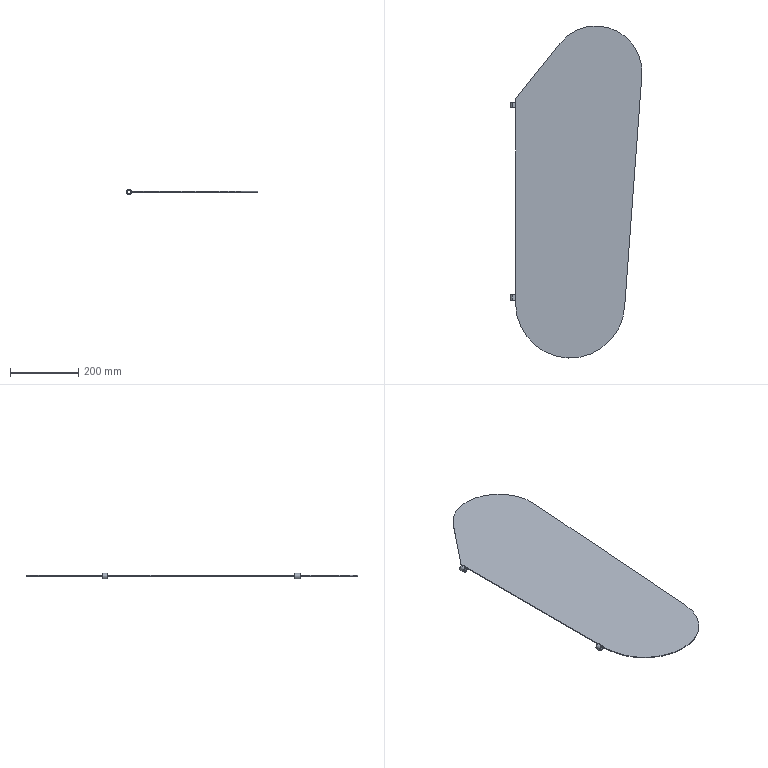Part | SolidWorks | features ICE 3, Extrusion 1, WeldmentFeature 1 | 3 solids | 19 faces | box 386.5 x 973.632 x 16 mm | volume 607839 mm3 | cylinder 10 | plane 9 | commonest cylinder face diameters 10 x4 16 x4 270 x1 320 x1
STEP:
#1=CARTESIAN_POINT('',(-185.,-325.,0.));
#2=VERTEX_POINT('',#1);
#3=CARTESIAN_POINT('',(134.56,-336.857,0.));
#4=VERTEX_POINT('',#3);
#5=CARTESIAN_POINT('',(-25.,-325.,0.));
#6=DIRECTION('',(0.,0.,1.));
#7=DIRECTION('',(1.,0.,0.));
#8=AXIS2_PLACEMENT_3D('',#5,#6,#7);
#9=CIRCLE('',#8,160.);
#10=EDGE_CURVE('',#2,#4,#9,.T.);
#11=ORIENTED_EDGE('',*,*,#10,.T.);
#12=CARTESIAN_POINT('',(134.56,-336.857,2.));
#13=VERTEX_POINT('',#12);
#14=CARTESIAN_POINT('',(134.56,-336.857,2.));
#15=DIRECTION('',(0.,0.,-1.));
#16=VECTOR('',#15,1000.);
#17=LINE('',#14,#16);
#18=EDGE_CURVE('',#13,#4,#17,.T.);
#19=ORIENTED_EDGE('',*,*,#18,.F.);
#20=CARTESIAN_POINT('',(-185.,-325.,2.));
#21=VERTEX_POINT('',#20);
#22=CARTESIAN_POINT('',(-25.,-325.,2.));
#23=DIRECTION('',(0.,0.,1.));
#24=DIRECTION('',(1.,0.,0.));
#25=AXIS2_PLACEMENT_3D('',#22,#23,#24);
#26=CIRCLE('',#25,160.);
#27=EDGE_CURVE('',#21,#13,#26,.T.);
#28=ORIENTED_EDGE('',*,*,#27,.F.);
#29=CARTESIAN_POINT('',(-185.,-325.,2.));
#30=DIRECTION('',(0.,0.,-1.));
#31=VECTOR('',#30,1000.);
#32=LINE('',#29,#31);
#33=EDGE_CURVE('',#21,#2,#32,.T.);
#34=ORIENTED_EDGE('',*,*,#33,.T.);
#35=EDGE_LOOP('',(#11,#19,#28,#34));
#36=FACE_OUTER_BOUND('',#35,.T.);
#37=CARTESIAN_POINT('',(-25.,-325.,2.));
#38=DIRECTION('',(0.,0.,-1.));
#39=DIRECTION('',(-1.,0.,0.));
#40=AXIS2_PLACEMENT_3D('',#37,#38,#39);
#41=CYLINDRICAL_SURFACE('',#40,160.);
#42=ADVANCED_FACE('',(#36),#41,.T.);
#43=CARTESIAN_POINT('',(185.129,343.627,0.));
#44=VERTEX_POINT('',#43);
#45=CARTESIAN_POINT('',(134.56,-336.857,0.));
#46=DIRECTION('',(0.07411,0.9973,0.));
#47=VECTOR('',#46,1000.);
#48=LINE('',#45,#47);
#49=EDGE_CURVE('',#4,#44,#48,.T.);
#50=ORIENTED_EDGE('',*,*,#49,.T.);
#51=CARTESIAN_POINT('',(185.129,343.627,2.));
#52=VERTEX_POINT('',#51);
#53=CARTESIAN_POINT('',(185.129,343.627,2.));
#54=DIRECTION('',(0.,0.,-1.));
#55=VECTOR('',#54,1000.);
#56=LINE('',#53,#55);
#57=EDGE_CURVE('',#52,#44,#56,.T.);
#58=ORIENTED_EDGE('',*,*,#57,.F.);
#59=CARTESIAN_POINT('',(134.56,-336.857,2.));
#60=DIRECTION('',(0.07411,0.9973,0.));
#61=VECTOR('',#60,1000.);
#62=LINE('',#59,#61);
#63=EDGE_CURVE('',#13,#52,#62,.T.);
#64=ORIENTED_EDGE('',*,*,#63,.F.);
#65=ORIENTED_EDGE('',*,*,#18,.T.);
#66=EDGE_LOOP('',(#50,#58,#64,#65));
#67=FACE_OUTER_BOUND('',#66,.T.);
#68=CARTESIAN_POINT('',(134.56,-336.857,2.));
#69=DIRECTION('',(-0.9973,0.07411,0.));
#70=DIRECTION('',(-0.07411,-0.9973,0.));
#71=AXIS2_PLACEMENT_3D('',#68,#69,#70);
#72=PLANE('',#71);
#73=ADVANCED_FACE('',(#67),#72,.F.);
#74=CARTESIAN_POINT('',(-55.009,437.851,0.));
#75=VERTEX_POINT('',#74);
#76=CARTESIAN_POINT('',(50.5,353.632,0.));
#77=DIRECTION('',(0.,0.,1.));
#78=DIRECTION('',(1.,0.,0.));
#79=AXIS2_PLACEMENT_3D('',#76,#77,#78);
#80=CIRCLE('',#79,135.);
#81=EDGE_CURVE('',#44,#75,#80,.T.);
#82=ORIENTED_EDGE('',*,*,#81,.T.);
#83=CARTESIAN_POINT('',(-55.009,437.851,2.));
#84=VERTEX_POINT('',#83);
#85=CARTESIAN_POINT('',(-55.009,437.851,2.));
#86=DIRECTION('',(0.,0.,-1.));
#87=VECTOR('',#86,1000.);
#88=LINE('',#85,#87);
#89=EDGE_CURVE('',#84,#75,#88,.T.);
#90=ORIENTED_EDGE('',*,*,#89,.F.);
#91=CARTESIAN_POINT('',(50.5,353.632,2.));
#92=DIRECTION('',(0.,0.,1.));
#93=DIRECTION('',(1.,0.,0.));
#94=AXIS2_PLACEMENT_3D('',#91,#92,#93);
#95=CIRCLE('',#94,135.);
#96=EDGE_CURVE('',#52,#84,#95,.T.);
#97=ORIENTED_EDGE('',*,*,#96,.F.);
#98=ORIENTED_EDGE('',*,*,#57,.T.);
#99=EDGE_LOOP('',(#82,#90,#97,#98));
#100=FACE_OUTER_BOUND('',#99,.T.);
#101=CARTESIAN_POINT('',(50.5,353.632,2.));
#102=DIRECTION('',(0.,0.,-1.));
#103=DIRECTION('',(-1.,0.,0.));
#104=AXIS2_PLACEMENT_3D('',#101,#102,#103);
#105=CYLINDRICAL_SURFACE('',#104,135.);
#106=ADVANCED_FACE('',(#100),#105,.T.);
#107=CARTESIAN_POINT('',(-185.,275.,0.));
#108=VERTEX_POINT('',#107);
#109=CARTESIAN_POINT('',(-55.009,437.851,0.));
#110=DIRECTION('',(-0.6238,-0.7815,0.));
#111=VECTOR('',#110,1000.);
#112=LINE('',#109,#111);
#113=EDGE_CURVE('',#75,#108,#112,.T.);
#114=ORIENTED_EDGE('',*,*,#113,.T.);
#115=CARTESIAN_POINT('',(-185.,275.,2.));
#116=VERTEX_POINT('',#115);
#117=CARTESIAN_POINT('',(-185.,275.,2.));
#118=DIRECTION('',(0.,0.,-1.));
#119=VECTOR('',#118,1000.);
#120=LINE('',#117,#119);
#121=EDGE_CURVE('',#116,#108,#120,.T.);
#122=ORIENTED_EDGE('',*,*,#121,.F.);
#123=CARTESIAN_POINT('',(-55.009,437.851,2.));
#124=DIRECTION('',(-0.6238,-0.7815,0.));
#125=VECTOR('',#124,1000.);
#126=LINE('',#123,#125);
#127=EDGE_CURVE('',#84,#116,#126,.T.);
#128=ORIENTED_EDGE('',*,*,#127,.F.);
#129=ORIENTED_EDGE('',*,*,#89,.T.);
#130=EDGE_LOOP('',(#114,#122,#128,#129));
#131=FACE_OUTER_BOUND('',#130,.T.);
#132=CARTESIAN_POINT('',(-55.009,437.851,2.));
#133=DIRECTION('',(0.7815,-0.6238,0.));
#134=DIRECTION('',(0.6238,0.7815,0.));
#135=AXIS2_PLACEMENT_3D('',#132,#133,#134);
#136=PLANE('',#135);
#137=ADVANCED_FACE('',(#131),#136,.F.);
#138=CARTESIAN_POINT('',(-185.,275.,0.));
#139=DIRECTION('',(0.,-1.,0.));
#140=VECTOR('',#139,1000.);
#141=LINE('',#138,#140);
#142=EDGE_CURVE('',#108,#2,#141,.T.);
#143=ORIENTED_EDGE('',*,*,#142,.T.);
#144=ORIENTED_EDGE('',*,*,#33,.F.);
#145=CARTESIAN_POINT('',(-185.,275.,2.));
#146=DIRECTION('',(0.,-1.,0.));
#147=VECTOR('',#146,1000.);
#148=LINE('',#145,#147);
#149=EDGE_CURVE('',#116,#21,#148,.T.);
#150=ORIENTED_EDGE('',*,*,#149,.F.);
#151=ORIENTED_EDGE('',*,*,#121,.T.);
#152=EDGE_LOOP('',(#143,#144,#150,#151));
#153=FACE_OUTER_BOUND('',#152,.T.);
#154=CARTESIAN_POINT('',(-185.,275.,2.));
#155=DIRECTION('',(1.,0.,0.));
#156=DIRECTION('',(0.,0.,-1.));
#157=AXIS2_PLACEMENT_3D('',#154,#155,#156);
#158=PLANE('',#157);
#159=ADVANCED_FACE('',(#153),#158,.F.);
#160=ORIENTED_EDGE('',*,*,#27,.T.);
#161=ORIENTED_EDGE('',*,*,#63,.T.);
#162=ORIENTED_EDGE('',*,*,#96,.T.);
#163=ORIENTED_EDGE('',*,*,#127,.T.);
#164=ORIENTED_EDGE('',*,*,#149,.T.);
#165=EDGE_LOOP('',(#160,#161,#162,#163,#164));
#166=FACE_OUTER_BOUND('',#165,.T.);
#167=CARTESIAN_POINT('',(-25.,-325.,2.));
#168=DIRECTION('',(0.,0.,1.));
#169=DIRECTION('',(1.,0.,0.));
#170=AXIS2_PLACEMENT_3D('',#167,#168,#169);
#171=PLANE('',#170);
#172=ADVANCED_FACE('',(#166),#171,.T.);
#173=ORIENTED_EDGE('',*,*,#10,.F.);
#174=ORIENTED_EDGE('',*,*,#142,.F.);
#175=ORIENTED_EDGE('',*,*,#113,.F.);
#176=ORIENTED_EDGE('',*,*,#81,.F.);
#177=ORIENTED_EDGE('',*,*,#49,.F.);
#178=EDGE_LOOP('',(#173,#174,#175,#176,#177));
#179=FACE_OUTER_BOUND('',#178,.T.);
#180=CARTESIAN_POINT('',(-25.,-325.,0.));
#181=DIRECTION('',(0.,0.,1.));
#182=DIRECTION('',(1.,0.,0.));
#183=AXIS2_PLACEMENT_3D('',#180,#181,#182);
#184=PLANE('',#183);
#185=ADVANCED_FACE('',(#179),#184,.F.);
#186=CLOSED_SHELL('',(#42,#73,#106,#137,#159,#172,#185));
#187=MANIFOLD_SOLID_BREP('',#186);
#188=CARTESIAN_POINT('',(-193.,-315.,-5.));
#189=VERTEX_POINT('',#188);
#190=CARTESIAN_POINT('',(-193.,-315.,5.));
#191=VERTEX_POINT('',#190);
#192=CARTESIAN_POINT('',(-193.,-315.,0.));
#193=DIRECTION('',(0.,1.,0.));
#194=DIRECTION('',(0.,0.,1.));
#195=AXIS2_PLACEMENT_3D('',#192,#193,#194);
#196=CIRCLE('',#195,5.);
#197=EDGE_CURVE('',#189,#191,#196,.T.);
#198=ORIENTED_EDGE('',*,*,#197,.F.);
#199=CARTESIAN_POINT('',(-193.,-300.,-5.));
#200=VERTEX_POINT('',#199);
#201=CARTESIAN_POINT('',(-193.,-485.,-5.));
#202=DIRECTION('',(0.,1.,0.));
#203=VECTOR('',#202,1000.);
#204=LINE('',#201,#203);
#205=EDGE_CURVE('',#189,#200,#204,.T.);
#206=ORIENTED_EDGE('',*,*,#205,.T.);
#207=CARTESIAN_POINT('',(-193.,-300.,5.));
#208=VERTEX_POINT('',#207);
#209=CARTESIAN_POINT('',(-193.,-300.,0.));
#210=DIRECTION('',(0.,1.,0.));
#211=DIRECTION('',(0.,0.,1.));
#212=AXIS2_PLACEMENT_3D('',#209,#210,#211);
#213=CIRCLE('',#212,5.);
#214=EDGE_CURVE('',#200,#208,#213,.T.);
#215=ORIENTED_EDGE('',*,*,#214,.T.);
#216=CARTESIAN_POINT('',(-193.,-485.,5.));
#217=DIRECTION('',(0.,1.,0.));
#218=VECTOR('',#217,1000.);
#219=LINE('',#216,#218);
#220=EDGE_CURVE('',#191,#208,#219,.T.);
#221=ORIENTED_EDGE('',*,*,#220,.F.);
#222=EDGE_LOOP('',(#198,#206,#215,#221));
#223=FACE_OUTER_BOUND('',#222,.T.);
#224=CARTESIAN_POINT('',(-193.,-485.,0.));
#225=DIRECTION('',(0.,1.,0.));
#226=DIRECTION('',(0.,0.,1.));
#227=AXIS2_PLACEMENT_3D('',#224,#225,#226);
#228=CYLINDRICAL_SURFACE('',#227,5.);
#229=ADVANCED_FACE('',(#223),#228,.F.);
#230=CARTESIAN_POINT('',(-193.,-300.,8.));
#231=VERTEX_POINT('',#230);
#232=CARTESIAN_POINT('',(-193.,-300.,-8.));
#233=VERTEX_POINT('',#232);
#234=CARTESIAN_POINT('',(-193.,-300.,0.));
#235=DIRECTION('',(0.,1.,0.));
#236=DIRECTION('',(0.,0.,1.));
#237=AXIS2_PLACEMENT_3D('',#234,#235,#236);
#238=CIRCLE('',#237,8.);
#239=EDGE_CURVE('',#231,#233,#238,.T.);
#240=ORIENTED_EDGE('',*,*,#239,.F.);
#241=CARTESIAN_POINT('',(-193.,-315.,8.));
#242=VERTEX_POINT('',#241);
#243=CARTESIAN_POINT('',(-193.,-300.,8.));
#244=DIRECTION('',(0.,-1.,0.));
#245=VECTOR('',#244,1000.);
#246=LINE('',#243,#245);
#247=EDGE_CURVE('',#231,#242,#246,.T.);
#248=ORIENTED_EDGE('',*,*,#247,.T.);
#249=CARTESIAN_POINT('',(-193.,-315.,-8.));
#250=VERTEX_POINT('',#249);
#251=CARTESIAN_POINT('',(-193.,-315.,0.));
#252=DIRECTION('',(0.,1.,0.));
#253=DIRECTION('',(0.,0.,1.));
#254=AXIS2_PLACEMENT_3D('',#251,#252,#253);
#255=CIRCLE('',#254,8.);
#256=EDGE_CURVE('',#242,#250,#255,.T.);
#257=ORIENTED_EDGE('',*,*,#256,.T.);
#258=CARTESIAN_POINT('',(-193.,-300.,-8.));
#259=DIRECTION('',(0.,-1.,0.));
#260=VECTOR('',#259,1000.);
#261=LINE('',#258,#260);
#262=EDGE_CURVE('',#233,#250,#261,.T.);
#263=ORIENTED_EDGE('',*,*,#262,.F.);
#264=EDGE_LOOP('',(#240,#248,#257,#263));
#265=FACE_OUTER_BOUND('',#264,.T.);
#266=CARTESIAN_POINT('',(-193.,-300.,0.));
#267=DIRECTION('',(0.,-1.,0.));
#268=DIRECTION('',(0.,0.,-1.));
#269=AXIS2_PLACEMENT_3D('',#266,#267,#268);
#270=CYLINDRICAL_SURFACE('',#269,8.);
#271=ADVANCED_FACE('',(#265),#270,.T.);
#272=ORIENTED_EDGE('',*,*,#247,.F.);
#273=CARTESIAN_POINT('',(-193.,-300.,0.));
#274=DIRECTION('',(0.,1.,0.));
#275=DIRECTION('',(0.,0.,1.));
#276=AXIS2_PLACEMENT_3D('',#273,#274,#275);
#277=CIRCLE('',#276,8.);
#278=EDGE_CURVE('',#233,#231,#277,.T.);
#279=ORIENTED_EDGE('',*,*,#278,.F.);
#280=ORIENTED_EDGE('',*,*,#262,.T.);
#281=CARTESIAN_POINT('',(-193.,-315.,0.));
#282=DIRECTION('',(0.,1.,0.));
#283=DIRECTION('',(0.,0.,1.));
#284=AXIS2_PLACEMENT_3D('',#281,#282,#283);
#285=CIRCLE('',#284,8.);
#286=EDGE_CURVE('',#250,#242,#285,.T.);
#287=ORIENTED_EDGE('',*,*,#286,.T.);
#288=EDGE_LOOP('',(#272,#279,#280,#287));
#289=FACE_OUTER_BOUND('',#288,.T.);
#290=CARTESIAN_POINT('',(-193.,-300.,0.));
#291=DIRECTION('',(0.,-1.,0.));
#292=DIRECTION('',(0.,0.,-1.));
#293=AXIS2_PLACEMENT_3D('',#290,#291,#292);
#294=CYLINDRICAL_SURFACE('',#293,8.);
#295=ADVANCED_FACE('',(#289),#294,.T.);
#296=CARTESIAN_POINT('',(-193.,-300.,0.));
#297=DIRECTION('',(0.,1.,0.));
#298=DIRECTION('',(0.,0.,1.));
#299=AXIS2_PLACEMENT_3D('',#296,#297,#298);
#300=CIRCLE('',#299,5.);
#301=EDGE_CURVE('',#208,#200,#300,.T.);
#302=ORIENTED_EDGE('',*,*,#301,.F.);
#303=ORIENTED_EDGE('',*,*,#214,.F.);
#304=EDGE_LOOP('',(#302,#303));
#305=FACE_BOUND('',#304,.T.);
#306=ORIENTED_EDGE('',*,*,#278,.T.);
#307=ORIENTED_EDGE('',*,*,#239,.T.);
#308=EDGE_LOOP('',(#306,#307));
#309=FACE_OUTER_BOUND('',#308,.T.);
#310=CARTESIAN_POINT('',(-193.,-300.,0.));
#311=DIRECTION('',(0.,1.,0.));
#312=DIRECTION('',(0.,0.,1.));
#313=AXIS2_PLACEMENT_3D('',#310,#311,#312);
#314=PLANE('',#313);
#315=ADVANCED_FACE('',(#305,#309),#314,.T.);
#316=CARTESIAN_POINT('',(-193.,-315.,0.));
#317=DIRECTION('',(0.,1.,0.));
#318=DIRECTION('',(0.,0.,1.));
#319=AXIS2_PLACEMENT_3D('',#316,#317,#318);
#320=CIRCLE('',#319,5.);
#321=EDGE_CURVE('',#191,#189,#320,.T.);
#322=ORIENTED_EDGE('',*,*,#321,.T.);
#323=ORIENTED_EDGE('',*,*,#197,.T.);
#324=EDGE_LOOP('',(#322,#323));
#325=FACE_BOUND('',#324,.T.);
#326=ORIENTED_EDGE('',*,*,#286,.F.);
#327=ORIENTED_EDGE('',*,*,#256,.F.);
#328=EDGE_LOOP('',(#326,#327));
#329=FACE_OUTER_BOUND('',#328,.T.);
#330=CARTESIAN_POINT('',(-193.,-315.,0.));
#331=DIRECTION('',(0.,1.,0.));
#332=DIRECTION('',(0.,0.,1.));
#333=AXIS2_PLACEMENT_3D('',#330,#331,#332);
#334=PLANE('',#333);
#335=ADVANCED_FACE('',(#325,#329),#334,.F.);
#336=ORIENTED_EDGE('',*,*,#205,.F.);
#337=ORIENTED_EDGE('',*,*,#321,.F.);
#338=ORIENTED_EDGE('',*,*,#220,.T.);
#339=ORIENTED_EDGE('',*,*,#301,.T.);
#340=EDGE_LOOP('',(#336,#337,#338,#339));
#341=FACE_OUTER_BOUND('',#340,.T.);
#342=CARTESIAN_POINT('',(-193.,-485.,0.));
#343=DIRECTION('',(0.,1.,0.));
#344=DIRECTION('',(0.,0.,1.));
#345=AXIS2_PLACEMENT_3D('',#342,#343,#344);
#346=CYLINDRICAL_SURFACE('',#345,5.);
#347=ADVANCED_FACE('',(#341),#346,.F.);
#348=CLOSED_SHELL('',(#229,#271,#295,#315,#335,#347));
#349=MANIFOLD_SOLID_BREP('',#348);
#350=CARTESIAN_POINT('',(-193.,249.3,-5.));
#351=VERTEX_POINT('',#350);
#352=CARTESIAN_POINT('',(-193.,249.3,5.));
#353=VERTEX_POINT('',#352);
#354=CARTESIAN_POINT('',(-193.,249.3,0.));
#355=DIRECTION('',(0.,1.,0.));
#356=DIRECTION('',(0.,0.,1.));
#357=AXIS2_PLACEMENT_3D('',#354,#355,#356);
#358=CIRCLE('',#357,5.);
#359=EDGE_CURVE('',#351,#353,#358,.T.);
#360=ORIENTED_EDGE('',*,*,#359,.F.);
#361=CARTESIAN_POINT('',(-193.,264.3,-5.));
#362=VERTEX_POINT('',#361);
#363=CARTESIAN_POINT('',(-193.,-485.,-5.));
#364=DIRECTION('',(0.,1.,0.));
#365=VECTOR('',#364,1000.);
#366=LINE('',#363,#365);
#367=EDGE_CURVE('',#351,#362,#366,.T.);
#368=ORIENTED_EDGE('',*,*,#367,.T.);
#369=CARTESIAN_POINT('',(-193.,264.3,5.));
#370=VERTEX_POINT('',#369);
#371=CARTESIAN_POINT('',(-193.,264.3,0.));
#372=DIRECTION('',(0.,1.,0.));
#373=DIRECTION('',(0.,0.,1.));
#374=AXIS2_PLACEMENT_3D('',#371,#372,#373);
#375=CIRCLE('',#374,5.);
#376=EDGE_CURVE('',#362,#370,#375,.T.);
#377=ORIENTED_EDGE('',*,*,#376,.T.);
#378=CARTESIAN_POINT('',(-193.,-485.,5.));
#379=DIRECTION('',(0.,1.,0.));
#380=VECTOR('',#379,1000.);
#381=LINE('',#378,#380);
#382=EDGE_CURVE('',#353,#370,#381,.T.);
#383=ORIENTED_EDGE('',*,*,#382,.F.);
#384=EDGE_LOOP('',(#360,#368,#377,#383));
#385=FACE_OUTER_BOUND('',#384,.T.);
#386=CARTESIAN_POINT('',(-193.,-485.,0.));
#387=DIRECTION('',(0.,1.,0.));
#388=DIRECTION('',(0.,0.,1.));
#389=AXIS2_PLACEMENT_3D('',#386,#387,#388);
#390=CYLINDRICAL_SURFACE('',#389,5.);
#391=ADVANCED_FACE('',(#385),#390,.F.);
#392=CARTESIAN_POINT('',(-193.,249.3,8.));
#393=VERTEX_POINT('',#392);
#394=CARTESIAN_POINT('',(-193.,249.3,-8.));
#395=VERTEX_POINT('',#394);
#396=CARTESIAN_POINT('',(-193.,249.3,0.));
#397=DIRECTION('',(0.,1.,0.));
#398=DIRECTION('',(0.,0.,1.));
#399=AXIS2_PLACEMENT_3D('',#396,#397,#398);
#400=CIRCLE('',#399,8.);
#401=EDGE_CURVE('',#393,#395,#400,.T.);
#402=ORIENTED_EDGE('',*,*,#401,.T.);
#403=CARTESIAN_POINT('',(-193.,264.3,-8.));
#404=VERTEX_POINT('',#403);
#405=CARTESIAN_POINT('',(-193.,249.3,-8.));
#406=DIRECTION('',(0.,1.,0.));
#407=VECTOR('',#406,1000.);
#408=LINE('',#405,#407);
#409=EDGE_CURVE('',#395,#404,#408,.T.);
#410=ORIENTED_EDGE('',*,*,#409,.T.);
#411=CARTESIAN_POINT('',(-193.,264.3,8.));
#412=VERTEX_POINT('',#411);
#413=CARTESIAN_POINT('',(-193.,264.3,0.));
#414=DIRECTION('',(0.,1.,0.));
#415=DIRECTION('',(0.,0.,1.));
#416=AXIS2_PLACEMENT_3D('',#413,#414,#415);
#417=CIRCLE('',#416,8.);
#418=EDGE_CURVE('',#412,#404,#417,.T.);
#419=ORIENTED_EDGE('',*,*,#418,.F.);
#420=CARTESIAN_POINT('',(-193.,249.3,8.));
#421=DIRECTION('',(0.,1.,0.));
#422=VECTOR('',#421,1000.);
#423=LINE('',#420,#422);
#424=EDGE_CURVE('',#393,#412,#423,.T.);
#425=ORIENTED_EDGE('',*,*,#424,.F.);
#426=EDGE_LOOP('',(#402,#410,#419,#425));
#427=FACE_OUTER_BOUND('',#426,.T.);
#428=CARTESIAN_POINT('',(-193.,249.3,0.));
#429=DIRECTION('',(0.,1.,0.));
#430=DIRECTION('',(0.,0.,1.));
#431=AXIS2_PLACEMENT_3D('',#428,#429,#430);
#432=CYLINDRICAL_SURFACE('',#431,8.);
#433=ADVANCED_FACE('',(#427),#432,.T.);
#434=ORIENTED_EDGE('',*,*,#409,.F.);
#435=CARTESIAN_POINT('',(-193.,249.3,0.));
#436=DIRECTION('',(0.,1.,0.));
#437=DIRECTION('',(0.,0.,1.));
#438=AXIS2_PLACEMENT_3D('',#435,#436,#437);
#439=CIRCLE('',#438,8.);
#440=EDGE_CURVE('',#395,#393,#439,.T.);
#441=ORIENTED_EDGE('',*,*,#440,.T.);
#442=ORIENTED_EDGE('',*,*,#424,.T.);
#443=CARTESIAN_POINT('',(-193.,264.3,0.));
#444=DIRECTION('',(0.,1.,0.));
#445=DIRECTION('',(0.,0.,1.));
#446=AXIS2_PLACEMENT_3D('',#443,#444,#445);
#447=CIRCLE('',#446,8.);
#448=EDGE_CURVE('',#404,#412,#447,.T.);
#449=ORIENTED_EDGE('',*,*,#448,.F.);
#450=EDGE_LOOP('',(#434,#441,#442,#449));
#451=FACE_OUTER_BOUND('',#450,.T.);
#452=CARTESIAN_POINT('',(-193.,249.3,0.));
#453=DIRECTION('',(0.,1.,0.));
#454=DIRECTION('',(0.,0.,1.));
#455=AXIS2_PLACEMENT_3D('',#452,#453,#454);
#456=CYLINDRICAL_SURFACE('',#455,8.);
#457=ADVANCED_FACE('',(#451),#456,.T.);
#458=CARTESIAN_POINT('',(-193.,249.3,0.));
#459=DIRECTION('',(0.,1.,0.));
#460=DIRECTION('',(0.,0.,1.));
#461=AXIS2_PLACEMENT_3D('',#458,#459,#460);
#462=CIRCLE('',#461,5.);
#463=EDGE_CURVE('',#353,#351,#462,.T.);
#464=ORIENTED_EDGE('',*,*,#463,.T.);
#465=ORIENTED_EDGE('',*,*,#359,.T.);
#466=EDGE_LOOP('',(#464,#465));
#467=FACE_BOUND('',#466,.T.);
#468=ORIENTED_EDGE('',*,*,#401,.F.);
#469=ORIENTED_EDGE('',*,*,#440,.F.);
#470=EDGE_LOOP('',(#468,#469));
#471=FACE_OUTER_BOUND('',#470,.T.);
#472=CARTESIAN_POINT('',(-193.,249.3,0.));
#473=DIRECTION('',(0.,1.,0.));
#474=DIRECTION('',(0.,0.,1.));
#475=AXIS2_PLACEMENT_3D('',#472,#473,#474);
#476=PLANE('',#475);
#477=ADVANCED_FACE('',(#467,#471),#476,.F.);
#478=CARTESIAN_POINT('',(-193.,264.3,0.));
#479=DIRECTION('',(0.,1.,0.));
#480=DIRECTION('',(0.,0.,1.));
#481=AXIS2_PLACEMENT_3D('',#478,#479,#480);
#482=CIRCLE('',#481,5.);
#483=EDGE_CURVE('',#370,#362,#482,.T.);
#484=ORIENTED_EDGE('',*,*,#483,.F.);
#485=ORIENTED_EDGE('',*,*,#376,.F.);
#486=EDGE_LOOP('',(#484,#485));
#487=FACE_BOUND('',#486,.T.);
#488=ORIENTED_EDGE('',*,*,#418,.T.);
#489=ORIENTED_EDGE('',*,*,#448,.T.);
#490=EDGE_LOOP('',(#488,#489));
#491=FACE_OUTER_BOUND('',#490,.T.);
#492=CARTESIAN_POINT('',(-193.,264.3,0.));
#493=DIRECTION('',(0.,1.,0.));
#494=DIRECTION('',(0.,0.,1.));
#495=AXIS2_PLACEMENT_3D('',#492,#493,#494);
#496=PLANE('',#495);
#497=ADVANCED_FACE('',(#487,#491),#496,.T.);
#498=ORIENTED_EDGE('',*,*,#367,.F.);
#499=ORIENTED_EDGE('',*,*,#463,.F.);
#500=ORIENTED_EDGE('',*,*,#382,.T.);
#501=ORIENTED_EDGE('',*,*,#483,.T.);
#502=EDGE_LOOP('',(#498,#499,#500,#501));
#503=FACE_OUTER_BOUND('',#502,.T.);
#504=CARTESIAN_POINT('',(-193.,-485.,0.));
#505=DIRECTION('',(0.,1.,0.));
#506=DIRECTION('',(0.,0.,1.));
#507=AXIS2_PLACEMENT_3D('',#504,#505,#506);
#508=CYLINDRICAL_SURFACE('',#507,5.);
#509=ADVANCED_FACE('',(#503),#508,.F.);
#510=CLOSED_SHELL('',(#391,#433,#457,#477,#497,#509));
#511=MANIFOLD_SOLID_BREP('',#510);
#512=CARTESIAN_POINT('',(0.,0.,0.));
#513=DIRECTION('',(0.,0.,1.));
#514=DIRECTION('',(1.,0.,0.));
#515=AXIS2_PLACEMENT_3D('',#512,#513,#514);
#516=(LENGTH_UNIT()NAMED_UNIT(*)SI_UNIT(.MILLI.,.METRE.));
#517=UNCERTAINTY_MEASURE_WITH_UNIT(LENGTH_MEASURE(0.00001),#516,'','');
#518=(NAMED_UNIT(*)PLANE_ANGLE_UNIT()SI_UNIT($,.RADIAN.));
#519=(NAMED_UNIT(*)SI_UNIT($,.STERADIAN.)SOLID_ANGLE_UNIT());
#520=(GEOMETRIC_REPRESENTATION_CONTEXT(3)GLOBAL_UNCERTAINTY_ASSIGNED_CONTEXT((#517))GLOBAL_UNIT_ASSIGNED_CONTEXT((#516,#518,#519))REPRESENTATION_CONTEXT('',''));
#521=ADVANCED_BREP_SHAPE_REPRESENTATION('',(#187,#349,#511,#515),#520);